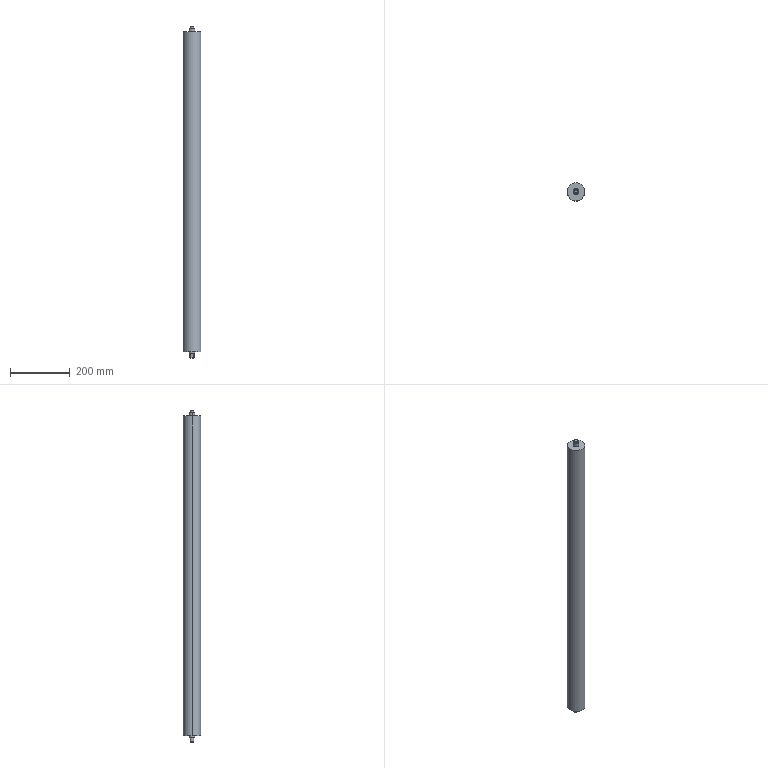Part | SolidWorks | features ICE 4, Chamfer 1, Revolution 1 | 1 solid | 26 faces | box 60 x 60 x 1111 mm | volume 3034450 mm3 | cylinder 11 | plane 10 | cone 5 | commonest cylinder face diameters 20 x4 15 x3 12 x2 60 x2
STEP:
#1=CARTESIAN_POINT('',(5.,0.,555.));
#2=VERTEX_POINT('',#1);
#3=CARTESIAN_POINT('',(-5.,0.,555.));
#4=VERTEX_POINT('',#3);
#5=CARTESIAN_POINT('',(0.,0.,555.));
#6=DIRECTION('',(0.,0.,1.));
#7=DIRECTION('',(1.,0.,0.));
#8=AXIS2_PLACEMENT_3D('',#5,#6,#7);
#9=CIRCLE('',#8,5.);
#10=EDGE_CURVE('',#2,#4,#9,.T.);
#11=ORIENTED_EDGE('',*,*,#10,.F.);
#12=CARTESIAN_POINT('',(6.,0.,554.));
#13=VERTEX_POINT('',#12);
#14=CARTESIAN_POINT('',(5.,0.,555.));
#15=DIRECTION('',(0.7071,0.,-0.7071));
#16=VECTOR('',#15,1000.);
#17=LINE('',#14,#16);
#18=EDGE_CURVE('',#2,#13,#17,.T.);
#19=ORIENTED_EDGE('',*,*,#18,.T.);
#20=CARTESIAN_POINT('',(-6.,0.,554.));
#21=VERTEX_POINT('',#20);
#22=CARTESIAN_POINT('',(0.,0.,554.));
#23=DIRECTION('',(0.,0.,-1.));
#24=DIRECTION('',(1.,0.,0.));
#25=AXIS2_PLACEMENT_3D('',#22,#23,#24);
#26=CIRCLE('',#25,6.);
#27=EDGE_CURVE('',#21,#13,#26,.T.);
#28=ORIENTED_EDGE('',*,*,#27,.F.);
#29=CARTESIAN_POINT('',(-5.,0.,555.));
#30=DIRECTION('',(-0.7071,0.,-0.7071));
#31=VECTOR('',#30,1000.);
#32=LINE('',#29,#31);
#33=EDGE_CURVE('',#4,#21,#32,.T.);
#34=ORIENTED_EDGE('',*,*,#33,.F.);
#35=EDGE_LOOP('',(#11,#19,#28,#34));
#36=FACE_OUTER_BOUND('',#35,.T.);
#37=CARTESIAN_POINT('',(0.,0.,555.));
#38=DIRECTION('',(0.,0.,-1.));
#39=DIRECTION('',(-1.,0.,0.));
#40=AXIS2_PLACEMENT_3D('',#37,#38,#39);
#41=CONICAL_SURFACE('',#40,5.,0.7854);
#42=ADVANCED_FACE('',(#36),#41,.T.);
#43=CARTESIAN_POINT('',(6.5,0.,-556.));
#44=VERTEX_POINT('',#43);
#45=CARTESIAN_POINT('',(4.153,-5.,-556.));
#46=VERTEX_POINT('',#45);
#47=CARTESIAN_POINT('',(0.,0.,-556.));
#48=DIRECTION('',(0.,0.,-1.));
#49=DIRECTION('',(1.,0.,0.));
#50=AXIS2_PLACEMENT_3D('',#47,#48,#49);
#51=CIRCLE('',#50,6.5);
#52=EDGE_CURVE('',#44,#46,#51,.T.);
#53=ORIENTED_EDGE('',*,*,#52,.F.);
#54=CARTESIAN_POINT('',(7.5,0.,-555.));
#55=VERTEX_POINT('',#54);
#56=CARTESIAN_POINT('',(6.5,0.,-556.));
#57=DIRECTION('',(0.7071,0.,0.7071));
#58=VECTOR('',#57,1000.);
#59=LINE('',#56,#58);
#60=EDGE_CURVE('',#44,#55,#59,.T.);
#61=ORIENTED_EDGE('',*,*,#60,.T.);
#62=CARTESIAN_POINT('',(4.5,-6.,-555.));
#63=VERTEX_POINT('',#62);
#64=CARTESIAN_POINT('',(0.,0.,-555.));
#65=DIRECTION('',(0.,0.,1.));
#66=DIRECTION('',(1.,0.,0.));
#67=AXIS2_PLACEMENT_3D('',#64,#65,#66);
#68=CIRCLE('',#67,7.5);
#69=EDGE_CURVE('',#63,#55,#68,.T.);
#70=ORIENTED_EDGE('',*,*,#69,.F.);
#71=CARTESIAN_POINT('',(4.5,-6.,-555.));
#72=CARTESIAN_POINT('',(4.389,-5.666,-555.334));
#73=CARTESIAN_POINT('',(4.273,-5.333,-555.667));
#74=CARTESIAN_POINT('',(4.153,-5.,-556.));
#75=B_SPLINE_CURVE_WITH_KNOTS('',3,(#71,#72,#73,#74),.UNSPECIFIED.,.F.,.F.,(4,4),(0.,0.001456),.UNSPECIFIED.);
#76=EDGE_CURVE('',#63,#46,#75,.T.);
#77=ORIENTED_EDGE('',*,*,#76,.T.);
#78=EDGE_LOOP('',(#53,#61,#70,#77));
#79=FACE_OUTER_BOUND('',#78,.T.);
#80=CARTESIAN_POINT('',(0.,0.,-556.));
#81=DIRECTION('',(0.,0.,1.));
#82=DIRECTION('',(1.,0.,0.));
#83=AXIS2_PLACEMENT_3D('',#80,#81,#82);
#84=CONICAL_SURFACE('',#83,6.5,0.7854);
#85=ADVANCED_FACE('',(#79),#84,.T.);
#86=ORIENTED_EDGE('',*,*,#27,.T.);
#87=CARTESIAN_POINT('',(6.,0.,548.));
#88=VERTEX_POINT('',#87);
#89=CARTESIAN_POINT('',(6.,0.,555.));
#90=DIRECTION('',(0.,0.,-1.));
#91=VECTOR('',#90,1000.);
#92=LINE('',#89,#91);
#93=EDGE_CURVE('',#13,#88,#92,.T.);
#94=ORIENTED_EDGE('',*,*,#93,.T.);
#95=CARTESIAN_POINT('',(-6.,0.,548.));
#96=VERTEX_POINT('',#95);
#97=CARTESIAN_POINT('',(0.,0.,548.));
#98=DIRECTION('',(0.,0.,1.));
#99=DIRECTION('',(1.,0.,0.));
#100=AXIS2_PLACEMENT_3D('',#97,#98,#99);
#101=CIRCLE('',#100,6.);
#102=EDGE_CURVE('',#88,#96,#101,.T.);
#103=ORIENTED_EDGE('',*,*,#102,.T.);
#104=CARTESIAN_POINT('',(-6.,0.,555.));
#105=DIRECTION('',(0.,0.,-1.));
#106=VECTOR('',#105,1000.);
#107=LINE('',#104,#106);
#108=EDGE_CURVE('',#21,#96,#107,.T.);
#109=ORIENTED_EDGE('',*,*,#108,.F.);
#110=EDGE_LOOP('',(#86,#94,#103,#109));
#111=FACE_OUTER_BOUND('',#110,.T.);
#112=CARTESIAN_POINT('',(0.,0.,555.));
#113=DIRECTION('',(0.,0.,-1.));
#114=DIRECTION('',(-1.,0.,0.));
#115=AXIS2_PLACEMENT_3D('',#112,#113,#114);
#116=CYLINDRICAL_SURFACE('',#115,6.);
#117=ADVANCED_FACE('',(#111),#116,.T.);
#118=CARTESIAN_POINT('',(10.,0.,548.));
#119=VERTEX_POINT('',#118);
#120=CARTESIAN_POINT('',(-10.,0.,548.));
#121=VERTEX_POINT('',#120);
#122=CARTESIAN_POINT('',(0.,0.,548.));
#123=DIRECTION('',(0.,0.,1.));
#124=DIRECTION('',(1.,0.,0.));
#125=AXIS2_PLACEMENT_3D('',#122,#123,#124);
#126=CIRCLE('',#125,10.);
#127=EDGE_CURVE('',#119,#121,#126,.T.);
#128=ORIENTED_EDGE('',*,*,#127,.F.);
#129=CARTESIAN_POINT('',(10.,0.,535.));
#130=VERTEX_POINT('',#129);
#131=CARTESIAN_POINT('',(10.,0.,548.));
#132=DIRECTION('',(0.,0.,-1.));
#133=VECTOR('',#132,1000.);
#134=LINE('',#131,#133);
#135=EDGE_CURVE('',#119,#130,#134,.T.);
#136=ORIENTED_EDGE('',*,*,#135,.T.);
#137=CARTESIAN_POINT('',(-10.,0.,535.));
#138=VERTEX_POINT('',#137);
#139=CARTESIAN_POINT('',(0.,0.,535.));
#140=DIRECTION('',(0.,0.,1.));
#141=DIRECTION('',(1.,0.,0.));
#142=AXIS2_PLACEMENT_3D('',#139,#140,#141);
#143=CIRCLE('',#142,10.);
#144=EDGE_CURVE('',#130,#138,#143,.T.);
#145=ORIENTED_EDGE('',*,*,#144,.T.);
#146=CARTESIAN_POINT('',(-10.,0.,548.));
#147=DIRECTION('',(0.,0.,-1.));
#148=VECTOR('',#147,1000.);
#149=LINE('',#146,#148);
#150=EDGE_CURVE('',#121,#138,#149,.T.);
#151=ORIENTED_EDGE('',*,*,#150,.F.);
#152=EDGE_LOOP('',(#128,#136,#145,#151));
#153=FACE_OUTER_BOUND('',#152,.T.);
#154=CARTESIAN_POINT('',(0.,0.,548.));
#155=DIRECTION('',(0.,0.,-1.));
#156=DIRECTION('',(-1.,0.,0.));
#157=AXIS2_PLACEMENT_3D('',#154,#155,#156);
#158=CYLINDRICAL_SURFACE('',#157,10.);
#159=ADVANCED_FACE('',(#153),#158,.T.);
#160=ORIENTED_EDGE('',*,*,#69,.T.);
#161=CARTESIAN_POINT('',(7.5,0.,-541.));
#162=VERTEX_POINT('',#161);
#163=CARTESIAN_POINT('',(7.5,0.,-556.));
#164=DIRECTION('',(0.,0.,1.));
#165=VECTOR('',#164,1000.);
#166=LINE('',#163,#165);
#167=EDGE_CURVE('',#55,#162,#166,.T.);
#168=ORIENTED_EDGE('',*,*,#167,.T.);
#169=CARTESIAN_POINT('',(4.5,-6.,-541.));
#170=VERTEX_POINT('',#169);
#171=CARTESIAN_POINT('',(0.,0.,-541.));
#172=DIRECTION('',(0.,0.,-1.));
#173=DIRECTION('',(1.,0.,0.));
#174=AXIS2_PLACEMENT_3D('',#171,#172,#173);
#175=CIRCLE('',#174,7.5);
#176=EDGE_CURVE('',#162,#170,#175,.T.);
#177=ORIENTED_EDGE('',*,*,#176,.T.);
#178=CARTESIAN_POINT('',(4.5,-6.,-556.));
#179=DIRECTION('',(0.,0.,1.));
#180=VECTOR('',#179,1000.);
#181=LINE('',#178,#180);
#182=EDGE_CURVE('',#63,#170,#181,.T.);
#183=ORIENTED_EDGE('',*,*,#182,.F.);
#184=EDGE_LOOP('',(#160,#168,#177,#183));
#185=FACE_OUTER_BOUND('',#184,.T.);
#186=CARTESIAN_POINT('',(0.,0.,-556.));
#187=DIRECTION('',(0.,0.,1.));
#188=DIRECTION('',(1.,0.,0.));
#189=AXIS2_PLACEMENT_3D('',#186,#187,#188);
#190=CYLINDRICAL_SURFACE('',#189,7.5);
#191=ADVANCED_FACE('',(#185),#190,.T.);
#192=CARTESIAN_POINT('',(-10.,0.,-541.));
#193=VERTEX_POINT('',#192);
#194=CARTESIAN_POINT('',(10.,0.,-541.));
#195=VERTEX_POINT('',#194);
#196=CARTESIAN_POINT('',(0.,0.,-541.));
#197=DIRECTION('',(0.,0.,-1.));
#198=DIRECTION('',(-1.,0.,0.));
#199=AXIS2_PLACEMENT_3D('',#196,#197,#198);
#200=CIRCLE('',#199,10.);
#201=EDGE_CURVE('',#193,#195,#200,.T.);
#202=ORIENTED_EDGE('',*,*,#201,.F.);
#203=CARTESIAN_POINT('',(-10.,0.,-535.));
#204=VERTEX_POINT('',#203);
#205=CARTESIAN_POINT('',(-10.,0.,-541.));
#206=DIRECTION('',(0.,0.,1.));
#207=VECTOR('',#206,1000.);
#208=LINE('',#205,#207);
#209=EDGE_CURVE('',#193,#204,#208,.T.);
#210=ORIENTED_EDGE('',*,*,#209,.T.);
#211=CARTESIAN_POINT('',(10.,0.,-535.));
#212=VERTEX_POINT('',#211);
#213=CARTESIAN_POINT('',(0.,0.,-535.));
#214=DIRECTION('',(0.,0.,-1.));
#215=DIRECTION('',(-1.,0.,0.));
#216=AXIS2_PLACEMENT_3D('',#213,#214,#215);
#217=CIRCLE('',#216,10.);
#218=EDGE_CURVE('',#204,#212,#217,.T.);
#219=ORIENTED_EDGE('',*,*,#218,.T.);
#220=CARTESIAN_POINT('',(10.,0.,-541.));
#221=DIRECTION('',(0.,0.,1.));
#222=VECTOR('',#221,1000.);
#223=LINE('',#220,#222);
#224=EDGE_CURVE('',#195,#212,#223,.T.);
#225=ORIENTED_EDGE('',*,*,#224,.F.);
#226=EDGE_LOOP('',(#202,#210,#219,#225));
#227=FACE_OUTER_BOUND('',#226,.T.);
#228=CARTESIAN_POINT('',(0.,0.,-541.));
#229=DIRECTION('',(0.,0.,1.));
#230=DIRECTION('',(1.,0.,0.));
#231=AXIS2_PLACEMENT_3D('',#228,#229,#230);
#232=CYLINDRICAL_SURFACE('',#231,10.);
#233=ADVANCED_FACE('',(#227),#232,.T.);
#234=CARTESIAN_POINT('',(-30.,0.,535.));
#235=VERTEX_POINT('',#234);
#236=CARTESIAN_POINT('',(30.,0.,535.));
#237=VERTEX_POINT('',#236);
#238=CARTESIAN_POINT('',(0.,0.,535.));
#239=DIRECTION('',(0.,0.,-1.));
#240=DIRECTION('',(-1.,0.,0.));
#241=AXIS2_PLACEMENT_3D('',#238,#239,#240);
#242=CIRCLE('',#241,30.);
#243=EDGE_CURVE('',#235,#237,#242,.T.);
#244=ORIENTED_EDGE('',*,*,#243,.T.);
#245=CARTESIAN_POINT('',(30.,0.,-535.));
#246=VERTEX_POINT('',#245);
#247=CARTESIAN_POINT('',(30.,0.,535.));
#248=DIRECTION('',(0.,0.,-1.));
#249=VECTOR('',#248,1000.);
#250=LINE('',#247,#249);
#251=EDGE_CURVE('',#237,#246,#250,.T.);
#252=ORIENTED_EDGE('',*,*,#251,.T.);
#253=CARTESIAN_POINT('',(-30.,0.,-535.));
#254=VERTEX_POINT('',#253);
#255=CARTESIAN_POINT('',(0.,0.,-535.));
#256=DIRECTION('',(0.,0.,-1.));
#257=DIRECTION('',(-1.,0.,0.));
#258=AXIS2_PLACEMENT_3D('',#255,#256,#257);
#259=CIRCLE('',#258,30.);
#260=EDGE_CURVE('',#254,#246,#259,.T.);
#261=ORIENTED_EDGE('',*,*,#260,.F.);
#262=CARTESIAN_POINT('',(-30.,0.,535.));
#263=DIRECTION('',(0.,0.,-1.));
#264=VECTOR('',#263,1000.);
#265=LINE('',#262,#264);
#266=EDGE_CURVE('',#235,#254,#265,.T.);
#267=ORIENTED_EDGE('',*,*,#266,.F.);
#268=EDGE_LOOP('',(#244,#252,#261,#267));
#269=FACE_OUTER_BOUND('',#268,.T.);
#270=CARTESIAN_POINT('',(0.,0.,535.));
#271=DIRECTION('',(0.,0.,-1.));
#272=DIRECTION('',(-1.,0.,0.));
#273=AXIS2_PLACEMENT_3D('',#270,#271,#272);
#274=CYLINDRICAL_SURFACE('',#273,30.);
#275=ADVANCED_FACE('',(#269),#274,.T.);
#276=ORIENTED_EDGE('',*,*,#251,.F.);
#277=CARTESIAN_POINT('',(0.,0.,535.));
#278=DIRECTION('',(0.,0.,-1.));
#279=DIRECTION('',(-1.,0.,0.));
#280=AXIS2_PLACEMENT_3D('',#277,#278,#279);
#281=CIRCLE('',#280,30.);
#282=EDGE_CURVE('',#237,#235,#281,.T.);
#283=ORIENTED_EDGE('',*,*,#282,.T.);
#284=ORIENTED_EDGE('',*,*,#266,.T.);
#285=CARTESIAN_POINT('',(0.,0.,-535.));
#286=DIRECTION('',(0.,0.,-1.));
#287=DIRECTION('',(-1.,0.,0.));
#288=AXIS2_PLACEMENT_3D('',#285,#286,#287);
#289=CIRCLE('',#288,30.);
#290=EDGE_CURVE('',#246,#254,#289,.T.);
#291=ORIENTED_EDGE('',*,*,#290,.F.);
#292=EDGE_LOOP('',(#276,#283,#284,#291));
#293=FACE_OUTER_BOUND('',#292,.T.);
#294=CARTESIAN_POINT('',(0.,0.,535.));
#295=DIRECTION('',(0.,0.,-1.));
#296=DIRECTION('',(-1.,0.,0.));
#297=AXIS2_PLACEMENT_3D('',#294,#295,#296);
#298=CYLINDRICAL_SURFACE('',#297,30.);
#299=ADVANCED_FACE('',(#293),#298,.T.);
#300=CARTESIAN_POINT('',(0.,0.,535.));
#301=DIRECTION('',(0.,0.,1.));
#302=DIRECTION('',(1.,0.,0.));
#303=AXIS2_PLACEMENT_3D('',#300,#301,#302);
#304=CIRCLE('',#303,10.);
#305=EDGE_CURVE('',#138,#130,#304,.T.);
#306=ORIENTED_EDGE('',*,*,#305,.F.);
#307=ORIENTED_EDGE('',*,*,#144,.F.);
#308=EDGE_LOOP('',(#306,#307));
#309=FACE_BOUND('',#308,.T.);
#310=ORIENTED_EDGE('',*,*,#243,.F.);
#311=ORIENTED_EDGE('',*,*,#282,.F.);
#312=EDGE_LOOP('',(#310,#311));
#313=FACE_OUTER_BOUND('',#312,.T.);
#314=CARTESIAN_POINT('',(30.,0.,535.));
#315=DIRECTION('',(0.,0.,1.));
#316=DIRECTION('',(1.,0.,0.));
#317=AXIS2_PLACEMENT_3D('',#314,#315,#316);
#318=PLANE('',#317);
#319=ADVANCED_FACE('',(#309,#313),#318,.T.);
#320=CARTESIAN_POINT('',(0.,0.,-535.));
#321=DIRECTION('',(0.,0.,-1.));
#322=DIRECTION('',(-1.,0.,0.));
#323=AXIS2_PLACEMENT_3D('',#320,#321,#322);
#324=CIRCLE('',#323,10.);
#325=EDGE_CURVE('',#212,#204,#324,.T.);
#326=ORIENTED_EDGE('',*,*,#325,.F.);
#327=ORIENTED_EDGE('',*,*,#218,.F.);
#328=EDGE_LOOP('',(#326,#327));
#329=FACE_BOUND('',#328,.T.);
#330=ORIENTED_EDGE('',*,*,#260,.T.);
#331=ORIENTED_EDGE('',*,*,#290,.T.);
#332=EDGE_LOOP('',(#330,#331));
#333=FACE_OUTER_BOUND('',#332,.T.);
#334=CARTESIAN_POINT('',(0.,0.,-535.));
#335=DIRECTION('',(0.,0.,-1.));
#336=DIRECTION('',(-1.,0.,0.));
#337=AXIS2_PLACEMENT_3D('',#334,#335,#336);
#338=PLANE('',#337);
#339=ADVANCED_FACE('',(#329,#333),#338,.T.);
#340=ORIENTED_EDGE('',*,*,#209,.F.);
#341=CARTESIAN_POINT('',(0.,0.,-541.));
#342=DIRECTION('',(0.,0.,-1.));
#343=DIRECTION('',(-1.,0.,0.));
#344=AXIS2_PLACEMENT_3D('',#341,#342,#343);
#345=CIRCLE('',#344,10.);
#346=EDGE_CURVE('',#195,#193,#345,.T.);
#347=ORIENTED_EDGE('',*,*,#346,.F.);
#348=ORIENTED_EDGE('',*,*,#224,.T.);
#349=ORIENTED_EDGE('',*,*,#325,.T.);
#350=EDGE_LOOP('',(#340,#347,#348,#349));
#351=FACE_OUTER_BOUND('',#350,.T.);
#352=CARTESIAN_POINT('',(0.,0.,-541.));
#353=DIRECTION('',(0.,0.,1.));
#354=DIRECTION('',(1.,0.,0.));
#355=AXIS2_PLACEMENT_3D('',#352,#353,#354);
#356=CYLINDRICAL_SURFACE('',#355,10.);
#357=ADVANCED_FACE('',(#351),#356,.T.);
#358=CARTESIAN_POINT('',(4.5,6.,-541.));
#359=VERTEX_POINT('',#358);
#360=CARTESIAN_POINT('',(0.,0.,-541.));
#361=DIRECTION('',(0.,0.,-1.));
#362=DIRECTION('',(1.,0.,0.));
#363=AXIS2_PLACEMENT_3D('',#360,#361,#362);
#364=CIRCLE('',#363,7.5);
#365=EDGE_CURVE('',#359,#162,#364,.T.);
#366=ORIENTED_EDGE('',*,*,#365,.F.);
#367=CARTESIAN_POINT('',(-4.5,6.,-541.));
#368=VERTEX_POINT('',#367);
#369=CARTESIAN_POINT('',(4.5,6.,-541.));
#370=DIRECTION('',(1.,0.,0.));
#371=VECTOR('',#370,1000.);
#372=LINE('',#369,#371);
#373=EDGE_CURVE('',#368,#359,#372,.T.);
#374=ORIENTED_EDGE('',*,*,#373,.F.);
#375=CARTESIAN_POINT('',(-4.5,-6.,-541.));
#376=VERTEX_POINT('',#375);
#377=CARTESIAN_POINT('',(0.,0.,-541.));
#378=DIRECTION('',(0.,0.,-1.));
#379=DIRECTION('',(1.,0.,0.));
#380=AXIS2_PLACEMENT_3D('',#377,#378,#379);
#381=CIRCLE('',#380,7.5);
#382=EDGE_CURVE('',#376,#368,#381,.T.);
#383=ORIENTED_EDGE('',*,*,#382,.F.);
#384=CARTESIAN_POINT('',(-4.5,-6.,-541.));
#385=DIRECTION('',(-1.,0.,0.));
#386=VECTOR('',#385,1000.);
#387=LINE('',#384,#386);
#388=EDGE_CURVE('',#170,#376,#387,.T.);
#389=ORIENTED_EDGE('',*,*,#388,.F.);
#390=ORIENTED_EDGE('',*,*,#176,.F.);
#391=EDGE_LOOP('',(#366,#374,#383,#389,#390));
#392=FACE_BOUND('',#391,.T.);
#393=ORIENTED_EDGE('',*,*,#346,.T.);
#394=ORIENTED_EDGE('',*,*,#201,.T.);
#395=EDGE_LOOP('',(#393,#394));
#396=FACE_OUTER_BOUND('',#395,.T.);
#397=CARTESIAN_POINT('',(0.,0.,-541.));
#398=DIRECTION('',(0.,0.,-1.));
#399=DIRECTION('',(-1.,0.,0.));
#400=AXIS2_PLACEMENT_3D('',#397,#398,#399);
#401=PLANE('',#400);
#402=ADVANCED_FACE('',(#392,#396),#401,.T.);
#403=ORIENTED_EDGE('',*,*,#167,.F.);
#404=CARTESIAN_POINT('',(4.5,6.,-555.));
#405=VERTEX_POINT('',#404);
#406=CARTESIAN_POINT('',(0.,0.,-555.));
#407=DIRECTION('',(0.,0.,1.));
#408=DIRECTION('',(1.,0.,0.));
#409=AXIS2_PLACEMENT_3D('',#406,#407,#408);
#410=CIRCLE('',#409,7.5);
#411=EDGE_CURVE('',#55,#405,#410,.T.);
#412=ORIENTED_EDGE('',*,*,#411,.T.);
#413=CARTESIAN_POINT('',(4.5,6.,-556.));
#414=DIRECTION('',(0.,0.,1.));
#415=VECTOR('',#414,1000.);
#416=LINE('',#413,#415);
#417=EDGE_CURVE('',#405,#359,#416,.T.);
#418=ORIENTED_EDGE('',*,*,#417,.T.);
#419=ORIENTED_EDGE('',*,*,#365,.T.);
#420=EDGE_LOOP('',(#403,#412,#418,#419));
#421=FACE_OUTER_BOUND('',#420,.T.);
#422=CARTESIAN_POINT('',(0.,0.,-556.));
#423=DIRECTION('',(0.,0.,1.));
#424=DIRECTION('',(1.,0.,0.));
#425=AXIS2_PLACEMENT_3D('',#422,#423,#424);
#426=CYLINDRICAL_SURFACE('',#425,7.5);
#427=ADVANCED_FACE('',(#421),#426,.T.);
#428=CARTESIAN_POINT('',(-4.5,-6.,-555.));
#429=VERTEX_POINT('',#428);
#430=CARTESIAN_POINT('',(-4.5,-6.,-556.));
#431=DIRECTION('',(0.,0.,1.));
#432=VECTOR('',#431,1000.);
#433=LINE('',#430,#432);
#434=EDGE_CURVE('',#429,#376,#433,.T.);
#435=ORIENTED_EDGE('',*,*,#434,.F.);
#436=CARTESIAN_POINT('',(-4.5,-6.,-555.));
#437=DIRECTION('',(1.,0.,0.));
#438=VECTOR('',#437,1000.);
#439=LINE('',#436,#438);
#440=EDGE_CURVE('',#429,#63,#439,.T.);
#441=ORIENTED_EDGE('',*,*,#440,.T.);
#442=ORIENTED_EDGE('',*,*,#182,.T.);
#443=ORIENTED_EDGE('',*,*,#388,.T.);
#444=EDGE_LOOP('',(#435,#441,#442,#443));
#445=FACE_OUTER_BOUND('',#444,.T.);
#446=CARTESIAN_POINT('',(-4.5,-6.,-556.));
#447=DIRECTION('',(0.,1.,0.));
#448=DIRECTION('',(-1.,0.,0.));
#449=AXIS2_PLACEMENT_3D('',#446,#447,#448);
#450=PLANE('',#449);
#451=ADVANCED_FACE('',(#445),#450,.F.);
#452=CARTESIAN_POINT('',(-4.5,6.,-555.));
#453=VERTEX_POINT('',#452);
#454=CARTESIAN_POINT('',(-4.5,6.,-556.));
#455=DIRECTION('',(0.,0.,1.));
#456=VECTOR('',#455,1000.);
#457=LINE('',#454,#456);
#458=EDGE_CURVE('',#453,#368,#457,.T.);
#459=ORIENTED_EDGE('',*,*,#458,.F.);
#460=CARTESIAN_POINT('',(0.,0.,-555.));
#461=DIRECTION('',(0.,0.,1.));
#462=DIRECTION('',(1.,0.,0.));
#463=AXIS2_PLACEMENT_3D('',#460,#461,#462);
#464=CIRCLE('',#463,7.5);
#465=EDGE_CURVE('',#453,#429,#464,.T.);
#466=ORIENTED_EDGE('',*,*,#465,.T.);
#467=ORIENTED_EDGE('',*,*,#434,.T.);
#468=ORIENTED_EDGE('',*,*,#382,.T.);
#469=EDGE_LOOP('',(#459,#466,#467,#468));
#470=FACE_OUTER_BOUND('',#469,.T.);
#471=CARTESIAN_POINT('',(0.,0.,-556.));
#472=DIRECTION('',(0.,0.,1.));
#473=DIRECTION('',(1.,0.,0.));
#474=AXIS2_PLACEMENT_3D('',#471,#472,#473);
#475=CYLINDRICAL_SURFACE('',#474,7.5);
#476=ADVANCED_FACE('',(#470),#475,.T.);
#477=ORIENTED_EDGE('',*,*,#417,.F.);
#478=CARTESIAN_POINT('',(4.5,6.,-555.));
#479=DIRECTION('',(-1.,0.,0.));
#480=VECTOR('',#479,1000.);
#481=LINE('',#478,#480);
#482=EDGE_CURVE('',#405,#453,#481,.T.);
#483=ORIENTED_EDGE('',*,*,#482,.T.);
#484=ORIENTED_EDGE('',*,*,#458,.T.);
#485=ORIENTED_EDGE('',*,*,#373,.T.);
#486=EDGE_LOOP('',(#477,#483,#484,#485));
#487=FACE_OUTER_BOUND('',#486,.T.);
#488=CARTESIAN_POINT('',(4.5,6.,-556.));
#489=DIRECTION('',(0.,-1.,0.));
#490=DIRECTION('',(1.,0.,0.));
#491=AXIS2_PLACEMENT_3D('',#488,#489,#490);
#492=PLANE('',#491);
#493=ADVANCED_FACE('',(#487),#492,.F.);
#494=CARTESIAN_POINT('',(-4.153,-5.,-556.));
#495=VERTEX_POINT('',#494);
#496=CARTESIAN_POINT('',(-4.153,5.,-556.));
#497=VERTEX_POINT('',#496);
#498=CARTESIAN_POINT('',(0.,0.,-556.));
#499=DIRECTION('',(0.,0.,-1.));
#500=DIRECTION('',(1.,0.,0.));
#501=AXIS2_PLACEMENT_3D('',#498,#499,#500);
#502=CIRCLE('',#501,6.5);
#503=EDGE_CURVE('',#495,#497,#502,.T.);
#504=ORIENTED_EDGE('',*,*,#503,.T.);
#505=CARTESIAN_POINT('',(4.153,5.,-556.));
#506=VERTEX_POINT('',#505);
#507=CARTESIAN_POINT('',(0.,5.,-556.));
#508=DIRECTION('',(1.,0.,0.));
#509=VECTOR('',#508,1000.);
#510=LINE('',#507,#509);
#511=EDGE_CURVE('',#497,#506,#510,.T.);
#512=ORIENTED_EDGE('',*,*,#511,.T.);
#513=CARTESIAN_POINT('',(0.,0.,-556.));
#514=DIRECTION('',(0.,0.,-1.));
#515=DIRECTION('',(1.,0.,0.));
#516=AXIS2_PLACEMENT_3D('',#513,#514,#515);
#517=CIRCLE('',#516,6.5);
#518=EDGE_CURVE('',#506,#44,#517,.T.);
#519=ORIENTED_EDGE('',*,*,#518,.T.);
#520=ORIENTED_EDGE('',*,*,#52,.T.);
#521=CARTESIAN_POINT('',(0.,-5.,-556.));
#522=DIRECTION('',(-1.,0.,0.));
#523=VECTOR('',#522,1000.);
#524=LINE('',#521,#523);
#525=EDGE_CURVE('',#46,#495,#524,.T.);
#526=ORIENTED_EDGE('',*,*,#525,.T.);
#527=EDGE_LOOP('',(#504,#512,#519,#520,#526));
#528=FACE_OUTER_BOUND('',#527,.T.);
#529=CARTESIAN_POINT('',(0.,0.,-556.));
#530=DIRECTION('',(0.,0.,1.));
#531=DIRECTION('',(1.,0.,0.));
#532=AXIS2_PLACEMENT_3D('',#529,#530,#531);
#533=PLANE('',#532);
#534=ADVANCED_FACE('',(#528),#533,.F.);
#535=ORIENTED_EDGE('',*,*,#135,.F.);
#536=CARTESIAN_POINT('',(0.,0.,548.));
#537=DIRECTION('',(0.,0.,1.));
#538=DIRECTION('',(1.,0.,0.));
#539=AXIS2_PLACEMENT_3D('',#536,#537,#538);
#540=CIRCLE('',#539,10.);
#541=EDGE_CURVE('',#121,#119,#540,.T.);
#542=ORIENTED_EDGE('',*,*,#541,.F.);
#543=ORIENTED_EDGE('',*,*,#150,.T.);
#544=ORIENTED_EDGE('',*,*,#305,.T.);
#545=EDGE_LOOP('',(#535,#542,#543,#544));
#546=FACE_OUTER_BOUND('',#545,.T.);
#547=CARTESIAN_POINT('',(0.,0.,548.));
#548=DIRECTION('',(0.,0.,-1.));
#549=DIRECTION('',(-1.,0.,0.));
#550=AXIS2_PLACEMENT_3D('',#547,#548,#549);
#551=CYLINDRICAL_SURFACE('',#550,10.);
#552=ADVANCED_FACE('',(#546),#551,.T.);
#553=CARTESIAN_POINT('',(0.,0.,548.));
#554=DIRECTION('',(0.,0.,1.));
#555=DIRECTION('',(1.,0.,0.));
#556=AXIS2_PLACEMENT_3D('',#553,#554,#555);
#557=CIRCLE('',#556,6.);
#558=EDGE_CURVE('',#96,#88,#557,.T.);
#559=ORIENTED_EDGE('',*,*,#558,.F.);
#560=ORIENTED_EDGE('',*,*,#102,.F.);
#561=EDGE_LOOP('',(#559,#560));
#562=FACE_BOUND('',#561,.T.);
#563=ORIENTED_EDGE('',*,*,#541,.T.);
#564=ORIENTED_EDGE('',*,*,#127,.T.);
#565=EDGE_LOOP('',(#563,#564));
#566=FACE_OUTER_BOUND('',#565,.T.);
#567=CARTESIAN_POINT('',(0.,0.,548.));
#568=DIRECTION('',(0.,0.,1.));
#569=DIRECTION('',(1.,0.,0.));
#570=AXIS2_PLACEMENT_3D('',#567,#568,#569);
#571=PLANE('',#570);
#572=ADVANCED_FACE('',(#562,#566),#571,.T.);
#573=ORIENTED_EDGE('',*,*,#93,.F.);
#574=CARTESIAN_POINT('',(0.,0.,554.));
#575=DIRECTION('',(0.,0.,-1.));
#576=DIRECTION('',(1.,0.,0.));
#577=AXIS2_PLACEMENT_3D('',#574,#575,#576);
#578=CIRCLE('',#577,6.);
#579=EDGE_CURVE('',#13,#21,#578,.T.);
#580=ORIENTED_EDGE('',*,*,#579,.T.);
#581=ORIENTED_EDGE('',*,*,#108,.T.);
#582=ORIENTED_EDGE('',*,*,#558,.T.);
#583=EDGE_LOOP('',(#573,#580,#581,#582));
#584=FACE_OUTER_BOUND('',#583,.T.);
#585=CARTESIAN_POINT('',(0.,0.,555.));
#586=DIRECTION('',(0.,0.,-1.));
#587=DIRECTION('',(-1.,0.,0.));
#588=AXIS2_PLACEMENT_3D('',#585,#586,#587);
#589=CYLINDRICAL_SURFACE('',#588,6.);
#590=ADVANCED_FACE('',(#584),#589,.T.);
#591=CARTESIAN_POINT('',(0.,0.,555.));
#592=DIRECTION('',(0.,0.,1.));
#593=DIRECTION('',(1.,0.,0.));
#594=AXIS2_PLACEMENT_3D('',#591,#592,#593);
#595=CIRCLE('',#594,5.);
#596=EDGE_CURVE('',#4,#2,#595,.T.);
#597=ORIENTED_EDGE('',*,*,#596,.T.);
#598=ORIENTED_EDGE('',*,*,#10,.T.);
#599=EDGE_LOOP('',(#597,#598));
#600=FACE_OUTER_BOUND('',#599,.T.);
#601=CARTESIAN_POINT('',(0.,0.,555.));
#602=DIRECTION('',(0.,0.,1.));
#603=DIRECTION('',(1.,0.,0.));
#604=AXIS2_PLACEMENT_3D('',#601,#602,#603);
#605=PLANE('',#604);
#606=ADVANCED_FACE('',(#600),#605,.T.);
#607=ORIENTED_EDGE('',*,*,#76,.F.);
#608=ORIENTED_EDGE('',*,*,#440,.F.);
#609=CARTESIAN_POINT('',(-4.153,-5.,-556.));
#610=CARTESIAN_POINT('',(-4.273,-5.333,-555.667));
#611=CARTESIAN_POINT('',(-4.389,-5.666,-555.334));
#612=CARTESIAN_POINT('',(-4.5,-6.,-555.));
#613=B_SPLINE_CURVE_WITH_KNOTS('',3,(#609,#610,#611,#612),.UNSPECIFIED.,.F.,.F.,(4,4),(0.,0.001456),.UNSPECIFIED.);
#614=EDGE_CURVE('',#495,#429,#613,.T.);
#615=ORIENTED_EDGE('',*,*,#614,.F.);
#616=ORIENTED_EDGE('',*,*,#525,.F.);
#617=EDGE_LOOP('',(#607,#608,#615,#616));
#618=FACE_OUTER_BOUND('',#617,.T.);
#619=CARTESIAN_POINT('',(0.,-5.,-556.));
#620=DIRECTION('',(0.,0.7071,0.7071));
#621=DIRECTION('',(-1.,0.,0.));
#622=AXIS2_PLACEMENT_3D('',#619,#620,#621);
#623=PLANE('',#622);
#624=ADVANCED_FACE('',(#618),#623,.F.);
#625=ORIENTED_EDGE('',*,*,#614,.T.);
#626=ORIENTED_EDGE('',*,*,#465,.F.);
#627=CARTESIAN_POINT('',(-4.153,5.,-556.));
#628=CARTESIAN_POINT('',(-4.273,5.333,-555.667));
#629=CARTESIAN_POINT('',(-4.389,5.666,-555.334));
#630=CARTESIAN_POINT('',(-4.5,6.,-555.));
#631=B_SPLINE_CURVE_WITH_KNOTS('',3,(#627,#628,#629,#630),.UNSPECIFIED.,.F.,.F.,(4,4),(0.,0.001456),.UNSPECIFIED.);
#632=EDGE_CURVE('',#497,#453,#631,.T.);
#633=ORIENTED_EDGE('',*,*,#632,.F.);
#634=ORIENTED_EDGE('',*,*,#503,.F.);
#635=EDGE_LOOP('',(#625,#626,#633,#634));
#636=FACE_OUTER_BOUND('',#635,.T.);
#637=CARTESIAN_POINT('',(0.,0.,-556.));
#638=DIRECTION('',(0.,0.,1.));
#639=DIRECTION('',(1.,0.,0.));
#640=AXIS2_PLACEMENT_3D('',#637,#638,#639);
#641=CONICAL_SURFACE('',#640,6.5,0.7854);
#642=ADVANCED_FACE('',(#636),#641,.T.);
#643=ORIENTED_EDGE('',*,*,#60,.F.);
#644=ORIENTED_EDGE('',*,*,#518,.F.);
#645=CARTESIAN_POINT('',(4.5,6.,-555.));
#646=CARTESIAN_POINT('',(4.389,5.666,-555.334));
#647=CARTESIAN_POINT('',(4.273,5.333,-555.667));
#648=CARTESIAN_POINT('',(4.153,5.,-556.));
#649=B_SPLINE_CURVE_WITH_KNOTS('',3,(#645,#646,#647,#648),.UNSPECIFIED.,.F.,.F.,(4,4),(0.,0.001456),.UNSPECIFIED.);
#650=EDGE_CURVE('',#405,#506,#649,.T.);
#651=ORIENTED_EDGE('',*,*,#650,.F.);
#652=ORIENTED_EDGE('',*,*,#411,.F.);
#653=EDGE_LOOP('',(#643,#644,#651,#652));
#654=FACE_OUTER_BOUND('',#653,.T.);
#655=CARTESIAN_POINT('',(0.,0.,-556.));
#656=DIRECTION('',(0.,0.,1.));
#657=DIRECTION('',(1.,0.,0.));
#658=AXIS2_PLACEMENT_3D('',#655,#656,#657);
#659=CONICAL_SURFACE('',#658,6.5,0.7854);
#660=ADVANCED_FACE('',(#654),#659,.T.);
#661=ORIENTED_EDGE('',*,*,#632,.T.);
#662=ORIENTED_EDGE('',*,*,#482,.F.);
#663=ORIENTED_EDGE('',*,*,#650,.T.);
#664=ORIENTED_EDGE('',*,*,#511,.F.);
#665=EDGE_LOOP('',(#661,#662,#663,#664));
#666=FACE_OUTER_BOUND('',#665,.T.);
#667=CARTESIAN_POINT('',(0.,5.,-556.));
#668=DIRECTION('',(0.,-0.7071,0.7071));
#669=DIRECTION('',(1.,0.,0.));
#670=AXIS2_PLACEMENT_3D('',#667,#668,#669);
#671=PLANE('',#670);
#672=ADVANCED_FACE('',(#666),#671,.F.);
#673=ORIENTED_EDGE('',*,*,#18,.F.);
#674=ORIENTED_EDGE('',*,*,#596,.F.);
#675=ORIENTED_EDGE('',*,*,#33,.T.);
#676=ORIENTED_EDGE('',*,*,#579,.F.);
#677=EDGE_LOOP('',(#673,#674,#675,#676));
#678=FACE_OUTER_BOUND('',#677,.T.);
#679=CARTESIAN_POINT('',(0.,0.,555.));
#680=DIRECTION('',(0.,0.,-1.));
#681=DIRECTION('',(-1.,0.,0.));
#682=AXIS2_PLACEMENT_3D('',#679,#680,#681);
#683=CONICAL_SURFACE('',#682,5.,0.7854);
#684=ADVANCED_FACE('',(#678),#683,.T.);
#685=CLOSED_SHELL('',(#42,#85,#117,#159,#191,#233,#275,#299,#319,#339,#357,#402,#427,#451,#476,#493,#534,#552,#572,#590,#606,#624,#642,#660,#672,#684));
#686=MANIFOLD_SOLID_BREP('',#685);
#687=CARTESIAN_POINT('',(0.,0.,0.));
#688=DIRECTION('',(0.,0.,1.));
#689=DIRECTION('',(1.,0.,0.));
#690=AXIS2_PLACEMENT_3D('',#687,#688,#689);
#691=(LENGTH_UNIT()NAMED_UNIT(*)SI_UNIT(.MILLI.,.METRE.));
#692=UNCERTAINTY_MEASURE_WITH_UNIT(LENGTH_MEASURE(0.00001),#691,'','');
#693=(NAMED_UNIT(*)PLANE_ANGLE_UNIT()SI_UNIT($,.RADIAN.));
#694=(NAMED_UNIT(*)SI_UNIT($,.STERADIAN.)SOLID_ANGLE_UNIT());
#695=(GEOMETRIC_REPRESENTATION_CONTEXT(3)GLOBAL_UNCERTAINTY_ASSIGNED_CONTEXT((#692))GLOBAL_UNIT_ASSIGNED_CONTEXT((#691,#693,#694))REPRESENTATION_CONTEXT('',''));
#696=ADVANCED_BREP_SHAPE_REPRESENTATION('',(#686,#690),#695);